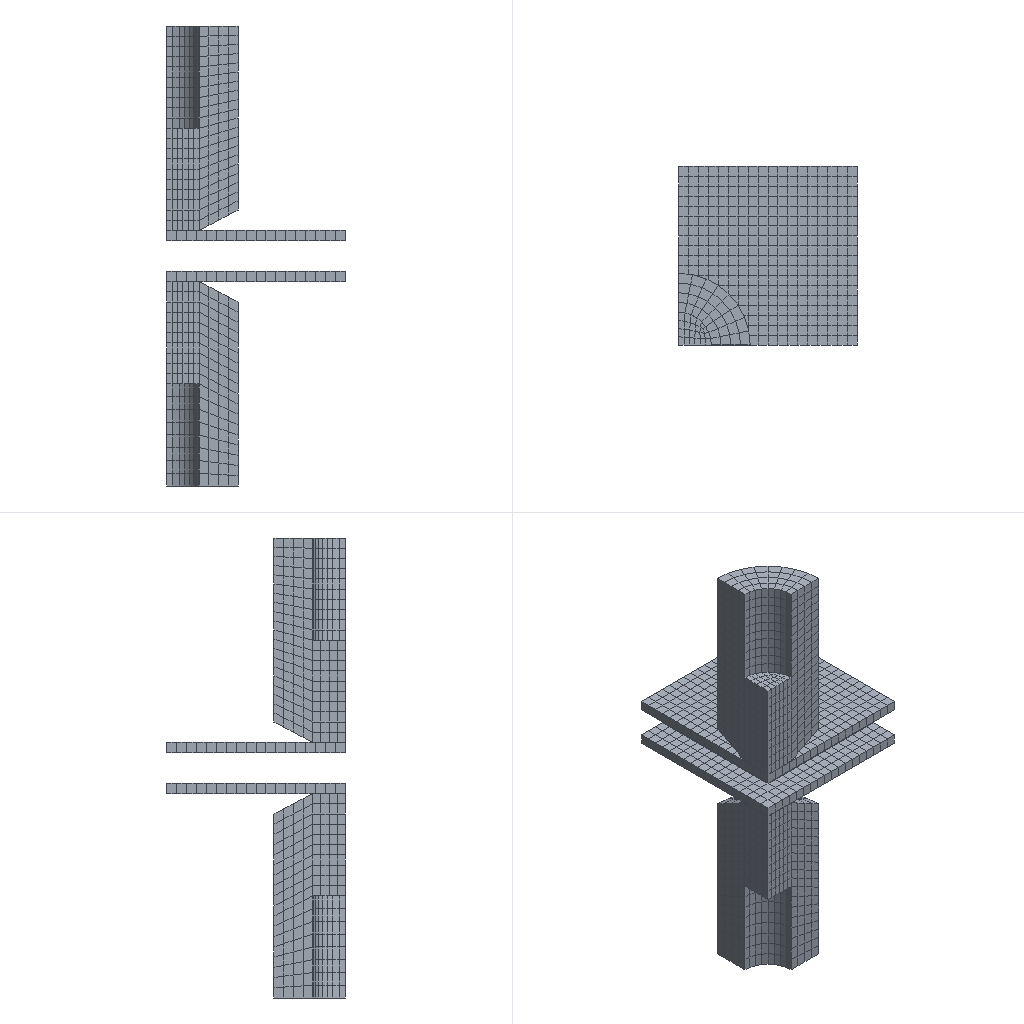Simulation study | abaqus
Set-up summary:
category,name,step,type,value,unit,region
solver,abaqus
solver,version,,,Abaqus/Standard 2020
units,not stated in the deck,,not stated
analysis,deck,,coupled temperature-displacement,coupled temperature-displacement
load_step,Step-1,Step-1,coupled temperature-displacement,nlgeom=True
load_step,Step-1-1,Step-1-1,coupled temperature-displacement,nlgeom=True
load_step,Step-2-jiazai,Step-2-jiazai,coupled temperature-displacement,nlgeom=True
load_step,Step-2-2-tongdian,Step-2-2-tongdian,coupled temperature-displacement,nlgeom=True
load_step,Step-2-3-xiezai,Step-2-3-xiezai,coupled temperature-displacement,nlgeom=True
load_step,Step-2-4-duandianbaochi,Step-2-4-duandianbaochi,coupled temperature-displacement,nlgeom=True
contact,interactions,,,general=0 pairs=3 ties=0
load_step,requested,,,6
mesh,nodes,,,3772
mesh,elements,,,2324
element_type,Q3D8R,,solid,2324
load,load commands in deck,,count,4
bc,support commands in deck,,count,25
material,CU_ELEC,,in results
material,FE_STEEL,,in results
check,setup vs results,,match,"per instance, exact: element labels, types and connectivity; labels of the nodes the elements use; coordinates of those nodes at SINGLE_PRECISION in 4 of 4 instance(s)"
Abaqus input file, long lists of numbers shortened:
*Heading
** Job name: Job-1 Model name: Job-model
** Generated by: Abaqus/CAE 2020
*Preprint, echo=NO, model=NO, history=NO, contact=NO
**
** PARTS
**
*Part, name=work-1
*Node
      1,           0.,   3.2,          14.
      2,           0.,           0.,          14.
** (1207 more lines like these left out)
*Element, type=Q3D8R
  1, 201, 202, 691, 684,  15,  16, 160, 159
  2, 202, 203, 692, 691,  16,  17, 161, 160
** (868 more lines like these left out)
*Nset, nset=Set-2, generate
    1,  1209,     1
*Elset, elset=Set-2, generate
   1,  870,    1
** Section: Section-2-SET-1
*Solid Section, elset=Set-2, material=CU_ELEC
,
*End Part
**
*Part, name=work-2
*Node
      1,         17.5,         17.5,           4.
      2,         17.5,         17.5,           3.
** (720 more lines like these left out)
*Element, type=Q3D8R
  1,  39,  40,  42,  41,   1,   2,   4,   3
  2,  41,  42,  44,  43,   3,   4,   6,   5
** (322 more lines like these left out)
*Nset, nset=Set-1, generate
   1,  722,    1
*Elset, elset=Set-1, generate
   1,  324,    1
** Section: Section-1-SET-1
*Solid Section, elset=Set-1, material=FE_STEEL
,
*End Part
**
*Part, name=work-3
*Node
      1,         17.5,         17.5,          -1.
      2,   16.528,         17.5,          -1.
** (720 more lines like these left out)
*Element, type=Q3D8R
  1,  39,  40,  59,  58,   1,   2,  21,  20
  2,  40,  41,  60,  59,   2,   3,  22,  21
** (322 more lines like these left out)
*Nset, nset=Set-1, generate
   1,  722,    1
*Elset, elset=Set-1, generate
   1,  324,    1
** Section: Section-1-SET-1
*Solid Section, elset=Set-1, material=FE_STEEL
,
*End Part
**
*Part, name=work-4
*Node
      1,           0.,   3.2,          -1.
      2,           0.,           0.,          -1.
** (1117 more lines like these left out)
*Element, type=Q3D8R
  1, 193, 194, 643, 636,  15,  16, 152, 151
  2, 194, 195, 644, 643,  16,  17, 153, 152
** (804 more lines like these left out)
*Nset, nset=Set-2, generate
    1,  1119,     1
*Elset, elset=Set-2, generate
   1,  806,    1
** Section: Section-4-SET-1
*Solid Section, elset=Set-2, material=CU_ELEC
,
*End Part
**
**
** ASSEMBLY
**
*Assembly, name=Assembly
**
*Instance, name=work-1-1, part=work-1
*End Instance
**
*Instance, name=work-2-1, part=work-2
*End Instance
**
*Instance, name=work-3-1, part=work-3
*End Instance
**
*Instance, name=work-4-1, part=work-4
*End Instance
**
*Nset, nset=Set-20, instance=work-1-1
   8,   9,  10,  11,  92,  93,  94, 111, 112, 113, 114, 115, 116, 117, 118, 119
 120, 121, 122, 123, 124, 134, 135, 136, 592, 593, 594, 595, 596, 597, 598, 599
** (1 more lines like these left out)
*Elset, elset=Set-20, instance=work-1-1
 307, 308, 309, 310, 387, 388, 389, 390, 467, 468, 469, 470, 547, 548, 549, 550
 627, 628, 629, 630, 707, 708, 709, 710, 787, 788, 789, 790, 867, 868, 869, 870
*Nset, nset=Set-21, instance=work-1-1
   2,   3,   5,   6,   7,   8,   9,  32,  33,  34,  35,  36,  37,  38,  39,  40
  41,  42,  43,  44,  45,  46,  47,  48,  49,  50,  51,  52,  53,  54,  65,  66
** (9 more lines like these left out)
*Nset, nset=Set-21, instance=work-2-1, generate
 685,  722,    1
*Nset, nset=Set-21, instance=work-4-1
   2,   3,   5,   6,   7,   8,   9,  32,  33,  34,  35,  36,  37,  38,  39,  40
  41,  42,  43,  44,  45,  46,  47,  48,  49,  50,  51,  52,  53,  54,  65,  66
** (9 more lines like these left out)
*Nset, nset=Set-21, instance=work-3-1, generate
 685,  722,    1
*Elset, elset=Set-21, instance=work-1-1
  28,  31,  34,  37,  40,  43,  46,  49,  52,  55,  58,  61,  64,  67,  70,  73
  76,  79,  82,  85,  88,  91,  94,  97, 100, 101, 104, 107, 110, 113, 143, 146
** (7 more lines like these left out)
*Elset, elset=Set-21, instance=work-2-1, generate
 307,  324,    1
*Elset, elset=Set-21, instance=work-4-1
  28,  31,  34,  37,  40,  43,  46,  49,  52,  55,  58,  61,  64,  67,  70,  73
  76,  79,  82,  85,  88,  91,  94,  97, 100, 101, 104, 107, 110, 113, 143, 146
** (7 more lines like these left out)
*Elset, elset=Set-21, instance=work-3-1, generate
 307,  324,    1
*Nset, nset=Set-22, instance=work-1-1
   1,   2,   4,   5,  10,  11,  12,  20,  21,  22,  23,  24,  25,  26,  27,  28
  29,  30,  31,  37,  38,  39,  40,  41,  42,  43,  44,  45,  55,  56,  57, 125
** (8 more lines like these left out)
*Nset, nset=Set-22, instance=work-2-1
  37,  38,  75,  76, 113, 114, 151, 152, 189, 190, 227, 228, 265, 266, 303, 304
 341, 342, 379, 380, 417, 418, 455, 456, 493, 494, 531, 532, 569, 570, 607, 608
** (1 more lines like these left out)
*Nset, nset=Set-22, instance=work-4-1
   1,   2,   4,   5,  10,  11,  12,  20,  21,  22,  23,  24,  25,  26,  27,  28
  29,  30,  31,  37,  38,  39,  40,  41,  42,  43,  44,  45,  55,  56,  57, 121
** (7 more lines like these left out)
*Nset, nset=Set-22, instance=work-3-1, generate
  19,  722,   19
*Elset, elset=Set-22, instance=work-1-1
   5,  10,  15,  20,  25,  26,  27,  28,  41,  42,  43,  56,  57,  58,  71,  72
  73,  86,  87,  88, 116, 117, 118, 119, 120, 141, 142, 143, 144, 145, 146, 147
** (6 more lines like these left out)
*Elset, elset=Set-22, instance=work-2-1, generate
  18,  324,   18
*Elset, elset=Set-22, instance=work-4-1
   5,  10,  15,  20,  25,  26,  27,  28,  41,  42,  43,  56,  57,  58,  71,  72
  73,  86,  87,  88, 116, 117, 118, 119, 120, 141, 142, 143, 144, 145, 146, 147
** (5 more lines like these left out)
*Elset, elset=Set-22, instance=work-3-1, generate
  18,  324,   18
*Nset, nset=Set-23, instance=work-2-1
   1,   2,  39,  40,  77,  78, 115, 116, 153, 154, 191, 192, 229, 230, 267, 268
 305, 306, 343, 344, 381, 382, 419, 420, 457, 458, 495, 496, 533, 534, 571, 572
** (1 more lines like these left out)
*Nset, nset=Set-23, instance=work-3-1, generate
   1,  704,   19
*Elset, elset=Set-23, instance=work-2-1, generate
   1,  307,   18
*Elset, elset=Set-23, instance=work-3-1, generate
   1,  307,   18
*Nset, nset=Set-24, instance=work-2-1, generate
  1,  38,   1
*Nset, nset=Set-24, instance=work-3-1, generate
  1,  38,   1
*Elset, elset=Set-24, instance=work-2-1, generate
  1,  18,   1
*Elset, elset=Set-24, instance=work-3-1, generate
  1,  18,   1
*Nset, nset=Set-25, instance=work-4-1
   7,   8,  11,  12,  77,  78,  79, 100, 101, 102, 103, 104, 105, 106, 107, 108
 109, 110, 111, 112, 113, 141, 142, 143, 467, 468, 469, 470, 471, 472, 473, 474
** (1 more lines like these left out)
*Elset, elset=Set-25, instance=work-4-1, generate
 248,  806,   18
*Nset, nset=Set-26, instance=work-1-1
   8,   9,  10,  11,  92,  93,  94, 111, 112, 113, 114, 115, 116, 117, 118, 119
 120, 121, 122, 123, 124, 134, 135, 136, 592, 593, 594, 595, 596, 597, 598, 599
** (1 more lines like these left out)
*Elset, elset=Set-26, instance=work-1-1
 307, 308, 309, 310, 387, 388, 389, 390, 467, 468, 469, 470, 547, 548, 549, 550
 627, 628, 629, 630, 707, 708, 709, 710, 787, 788, 789, 790, 867, 868, 869, 870
*Nset, nset=Set-27, instance=work-1-1
   8,   9,  10,  11,  92,  93,  94, 111, 112, 113, 114, 115, 116, 117, 118, 119
 120, 121, 122, 123, 124, 134, 135, 136, 592, 593, 594, 595, 596, 597, 598, 599
** (1 more lines like these left out)
*Nset, nset=Set-27, instance=work-4-1
   7,   8,  11,  12,  77,  78,  79, 100, 101, 102, 103, 104, 105, 106, 107, 108
 109, 110, 111, 112, 113, 141, 142, 143, 467, 468, 469, 470, 471, 472, 473, 474
** (1 more lines like these left out)
*Elset, elset=Set-27, instance=work-1-1
 307, 308, 309, 310, 387, 388, 389, 390, 467, 468, 469, 470, 547, 548, 549, 550
 627, 628, 629, 630, 707, 708, 709, 710, 787, 788, 789, 790, 867, 868, 869, 870
*Elset, elset=Set-27, instance=work-4-1, generate
 248,  806,   18
*Nset, nset=Set-28, instance=work-2-1
   1,   2,   3,   4,   5,   6,   7,   8,   9,  10,  11,  12,  13,  14,  15,  16
  17,  18,  19,  20,  21,  22,  23,  24,  25,  26,  27,  28,  29,  30,  31,  32
** (3 more lines like these left out)
*Nset, nset=Set-28, instance=work-3-1
   1,   2,   3,   4,   5,   6,   7,   8,   9,  10,  11,  12,  13,  14,  15,  16
  17,  18,  19,  20,  21,  22,  23,  24,  25,  26,  27,  28,  29,  30,  31,  32
** (3 more lines like these left out)
*Elset, elset=Set-28, instance=work-2-1
   1,   2,   3,   4,   5,   6,   7,   8,   9,  10,  11,  12,  13,  14,  15,  16
  17,  18,  19,  37,  55,  73,  91, 109, 127, 145, 163, 181, 199, 217, 235, 253
** (1 more lines like these left out)
*Elset, elset=Set-28, instance=work-3-1
   1,   2,   3,   4,   5,   6,   7,   8,   9,  10,  11,  12,  13,  14,  15,  16
  17,  18,  19,  37,  55,  73,  91, 109, 127, 145, 163, 181, 199, 217, 235, 253
** (1 more lines like these left out)
*Nset, nset=Set-29, instance=work-1-1, generate
    1,  1209,     1
*Nset, nset=Set-29, instance=work-2-1, generate
   1,  722,    1
*Nset, nset=Set-29, instance=work-4-1, generate
    1,  1119,     1
*Nset, nset=Set-29, instance=work-3-1, generate
   1,  722,    1
*Elset, elset=Set-29, instance=work-1-1, generate
   1,  870,    1
*Elset, elset=Set-29, instance=work-2-1, generate
   1,  324,    1
*Elset, elset=Set-29, instance=work-4-1, generate
   1,  806,    1
*Elset, elset=Set-29, instance=work-3-1, generate
   1,  324,    1
*Nset, nset=Set-30, instance=work-1-1
   1,   2,   3,  13,  14,  15,  16,  17,  18,  19,  20,  21,  22,  32,  33,  34
  35,  36, 159, 160, 161, 162, 163, 164, 165, 166, 167, 168, 169, 170, 171, 172
** (1 more lines like these left out)
*Elset, elset=Set-30, instance=work-1-1
   1,   2,   3,   4,   5,  26,  27,  28,  29,  30,  31,  32,  33,  34,  35,  36
  37,  38,  39,  40, 101, 102, 103
*Nset, nset=Set-31, instance=work-4-1
   4,   5,   6,  55,  56,  57,  58,  59,  60,  61,  62,  63,  64,  65,  66,  67
  68,  69, 301, 302, 303, 304, 305, 306, 307, 308, 309, 310, 311, 312, 313, 314
** (1 more lines like these left out)
*Elset, elset=Set-31, instance=work-4-1
 120, 125, 130, 135, 140, 141, 142, 143, 156, 157, 158, 171, 172, 173, 186, 187
 188, 201, 202, 203, 220, 225, 230
*Elset, elset=_Surf-6_S3, internal, instance=work-1-1
 307, 308, 309, 310, 387, 388, 389, 390, 467, 468, 469, 470, 547, 548, 549, 550
 627, 628, 629, 630, 707, 708, 709, 710, 787, 788, 789, 790, 867, 868, 869, 870
*Surface, type=ELEMENT, name=Surf-6
_Surf-6_S3, S3
*Elset, elset=_Surf-13_S3, internal, instance=work-1-1
 307, 308, 309, 310, 387, 388, 389, 390, 467, 468, 469, 470, 547, 548, 549, 550
 627, 628, 629, 630, 707, 708, 709, 710, 787, 788, 789, 790, 867, 868, 869, 870
*Elset, elset=_Surf-13_S4, internal, instance=work-4-1, generate
 248,  806,   18
*Surface, type=ELEMENT, name=Surf-13
_Surf-13_S3, S3
_Surf-13_S4, S4
*Elset, elset=_m_Surf-7_S4, internal, instance=work-2-1, generate
   1,  324,    1
*Surface, type=ELEMENT, name=m_Surf-7
_m_Surf-7_S4, S4
*Elset, elset=_m_Surf-9_S4, internal, instance=work-1-1
 120, 125, 130, 135, 140, 220, 225, 230
*Elset, elset=_m_Surf-9_S3, internal, instance=work-1-1
 141, 142, 143, 156, 157, 158, 171, 172, 173, 186, 187, 188, 201, 202, 203
*Elset, elset=_m_Surf-9_S5, internal, instance=work-1-1
 231, 232, 233, 234, 311, 312, 313, 314, 391, 392, 393, 394, 471, 472, 473, 474
 551, 552, 553, 554, 631, 632, 633, 634, 711, 712, 713, 714, 791, 792, 793, 794
*Surface, type=ELEMENT, name=m_Surf-9
_m_Surf-9_S4, S4
_m_Surf-9_S3, S3
_m_Surf-9_S5, S5
*Elset, elset=_m_Surf-11_S2, internal, instance=work-4-1
   1,   2,   3,   4,   5,  26,  27,  28,  29,  30,  31,  32,  33,  34,  35,  36
  37,  38,  39,  40, 101, 102, 103
*Elset, elset=_m_Surf-11_S6, internal, instance=work-4-1, generate
 231,  789,   18
*Surface, type=ELEMENT, name=m_Surf-11
_m_Surf-11_S2, S2
_m_Surf-11_S6, S6
*Elset, elset=_s_Surf-7_S5, internal, instance=work-3-1, generate
   1,  324,    1
*Surface, type=ELEMENT, name=s_Surf-7
_s_Surf-7_S5, S5
*Elset, elset=_s_Surf-9_S6, internal, instance=work-2-1, generate
   1,  324,    1
*Surface, type=ELEMENT, name=s_Surf-9
_s_Surf-9_S6, S6
*Elset, elset=_s_Surf-11_S3, internal, instance=work-3-1, generate
   1,  324,    1
*Surface, type=ELEMENT, name=s_Surf-11
_s_Surf-11_S3, S3
*End Assembly
*Amplitude, name=CURRENT_SHIJIA
             0.,              0.,            0.01,              1.
*Amplitude, name=CURRENT_XIEZAI
             0.,              1.,            0.01,              0.
*Amplitude, name=FORCE_SHIJIA
             0.,              0.,             0.1,              1.
*Amplitude, name=FORCE_XIEZAI
             0.,              1.,             0.1,              0.
**
** MATERIALS
**
*Material, name=CU_ELEC
*Conductivity
  385.,  25.
 368.5, 100.
 358.3, 210.
 342.1, 310.
 331.5, 430.
 319.6, 520.
 306.4, 630.
 298.1, 730.
 291.2, 850.
 288.6, 940.
 286.7,1030.
 282.5,1380.
*Density
 8.9e-09,
*Elastic
115000., 0.35,  20.
106000., 0.35, 150.
 99000., 0.36, 350.
 95000., 0.37, 450.
 87000., 0.37, 550.
 76000., 0.39, 650.
 71000., 0.39, 730.
*Electrical Conductivity
 28.41,  25.
   25., 110.
 18.75, 210.
 14.85, 310.
 13.32, 420.
 12.38, 530.
  9.02, 640.
  3.92, 750.
   3.4, 830.
  2.88, 950.
  2.37,1100.
  4.31,1220.
  3.92,1400.
*Expansion
 1.63e-05, 20.
 1.73e-05,150.
  1.8e-05,350.
 1.81e-05,450.
 1.86e-05,550.
 1.88e-05,650.
 1.94e-05,730.
*Joule Heat Fraction
         0.7,
*Plastic
233.,  0., 20.
188.,  0.,150.
130.,  0.,350.
125.,  0.,450.
107.,  0.,550.
 88.,  0.,650.
 50.,  0.,730.
*Specific Heat
 3.8e+08,  25.
 3.9e+08, 100.
   4e+08, 210.
 4.1e+08, 310.
 4.3e+08, 430.
 4.3e+08, 520.
 4.5e+08, 630.
 4.6e+08, 730.
 4.8e+08, 850.
 4.9e+08, 940.
 5.1e+08,1030.
 5.3e+08,1380.
*Material, name=FE_STEEL
*Conductivity
  15.6,  25.
 16.53, 100.
 17.89, 210.
 19.13, 310.
 20.62, 430.
 21.73, 520.
 23.09, 630.
 24.33, 730.
 25.81, 850.
 26.87, 940.
  27.9,1030.
 32.42,1380.
*Density
 7.8e-09,
*Elastic
205000.,  0.3,  20.
182000.,  0.3, 150.
169000.,  0.3, 350.
151000.,  0.3, 550.
121000.,  0.3, 750.
 75000.,  0.3, 950.
 46000.,  0.3,1300.
*Electrical Conductivity
 1.61,  25.
 1.33, 110.
 1.14, 210.
 1.01, 310.
 0.91, 420.
 0.84, 530.
 0.78, 640.
 0.74, 750.
 0.71, 830.
 0.68, 950.
 0.64,1100.
 0.62,1220.
  0.6,1400.
*Expansion
 2.023e-05,  20.
 2.046e-05, 150.
 2.087e-05, 350.
  2.13e-05, 550.
 2.178e-05, 750.
 2.238e-05, 950.
 2.341e-05,1300.
*Joule Heat Fraction
          1.,
*Plastic
300.,   0.,  20.
223.,   0., 150.
173.,   0., 350.
126.,   0., 550.
 95.,   0., 750.
 54.,   0., 950.
 32.,   0.,1300.
*Specific Heat
 4.6e+08,  25.
 4.8e+08, 100.
   5e+08, 210.
 5.2e+08, 310.
 5.4e+08, 430.
 5.5e+08, 520.
 5.7e+08, 630.
 5.9e+08, 730.
 6.1e+08, 850.
 6.8e+08, 940.
 6.5e+08,1030.
 8.8e+08,1380.
**
** INTERACTION PROPERTIES
**
*Surface Interaction, name=BAN_BAN
1.,
*Friction, slip tolerance=0.005
 0.2,
*Surface Behavior, pressure-overclosure=HARD
*Gap Conductance
140.,    0.,   20.
  0., 0.001,   20.
150.,    0.,  205.
  0., 0.001,  205.
160.,    0.,  650.
  0., 0.001,  650.
160.,    0.,  870.
  0., 0.001,  870.
*Gap Heat Generation
1., 0.5
*Gap Electrical Conductance
100.,   0.
  0., 0.01
*Surface Interaction, name=DJ_BAN
1.,
*Friction, slip tolerance=0.005
 0.2,
*Surface Behavior, pressure-overclosure=HARD
*Gap Conductance
 560.,    0.,   20.
   0., 0.001,   20.
 640.,    0.,  205.
   0., 0.001,  205.
1300.,    0.,  650.
   0., 0.001,  650.
4800.,    0.,  870.
   0., 0.001,  870.
*Gap Heat Generation
1., 0.5
*Gap Electrical Conductance
100.,   0.
  0., 0.01
**
** PHYSICAL CONSTANTS
**
*Physical Constants, absolute zero=-273.15, stefan boltzmann=5.67e-11
**
** BOUNDARY CONDITIONS
**
** Name: Disp-BC-1 Type: 对称/反对称/完全固定
*Boundary
Set-21, YSYMM
** Name: Disp-BC-2 Type: 对称/反对称/完全固定
*Boundary
Set-22, XSYMM
** Name: Disp-BC-3 Type: 位移/转角
*Boundary
Set-27, 1, 1
** Name: Disp-BC-8 Type: 位移/转角
*Boundary
Set-28, 1, 1
**
** PREDEFINED FIELDS
**
** Name: Predefined Field-1   Type: Temperature
*Initial Conditions, type=TEMPERATURE
Set-29, 20.
**
** INTERACTIONS
**
** Interaction: BAN_BAN-1
*Contact Pair, interaction=BAN_BAN, type=SURFACE TO SURFACE
s_Surf-7, m_Surf-7
** Interaction: Int-6
*Contact Pair, interaction=DJ_BAN, type=SURFACE TO SURFACE
m_Surf-9, s_Surf-9
** Interaction: Int-7
*Contact Pair, interaction=DJ_BAN, type=SURFACE TO SURFACE
s_Surf-11, m_Surf-11
** ----------------------------------------------------------------
**
** STEP: Step-1
**
*Step, name=Step-1, nlgeom=YES, inc=10000
*Coupled Temperature-displacement, electrical, creep=none, deltmx=1e+09
0.0015, 0.15, 1.5e-08, 0.015
**
** BOUNDARY CONDITIONS
**
** Name: Disp-BC-3 Type: 位移/转角
*Boundary
Set-27, 2, 2
Set-27, 4, 4
Set-27, 5, 5
Set-27, 6, 6
** Name: Disp-BC-8 Type: 位移/转角
*Boundary
Set-28, 2, 2
Set-28, 3, 3
**
** LOADS
**
** Name: Load-1   Type: Pressure
*Dsload, amplitude=FORCE_SHIJIA
Surf-13, P, 36.492
**
** OUTPUT REQUESTS
**
*Restart, write, frequency=0
**
** FIELD OUTPUT: F-Output-1
**
*Output, field
*Node Output
CECHG, CECUR, CF, EPOT, NT, RCHG, RECUR, RF
RFL, RM, RT, TF, U
*Element Output, directions=YES
E, ECD, EFLX, EPG, HFL, LE, MISES, MISESMAX, MISESONLY, NCURS, NE, P, PE, PEEQ, PEEQMAX, PEEQT
PEMAG, PRESSONLY, S, SEQUT, SF, SSAVG, TEMP, VEEQ, YIELDPOT
*Contact Output
CDISP, CSTRESS, ECD, ECDA, ECDT, ECDTA
*Radiation Output
FTEMP,
**
** HISTORY OUTPUT: H-Output-1
**
*Output, history, variable=PRESELECT
*End Step
** ----------------------------------------------------------------
**
** STEP: Step-1-1
**
*Step, name=Step-1-1, nlgeom=YES
*Coupled Temperature-displacement, electrical, creep=none, deltmx=1e+09
0.01, 0.3, 3e-06, 0.1
**
** LOADS
**
** Name: Load-1   Type: Pressure
**
** OUTPUT REQUESTS
**
*Restart, write, frequency=0
**
** FIELD OUTPUT: F-Output-1
**
*Output, field
*Node Output
CECHG, CECUR, CF, EPOT, NT, RCHG, RECUR, RF
RFL, RM, RT, TF, U
*Element Output, directions=YES
E, ECD, EFLX, EPG, HFL, LE, MISES, MISESMAX, MISESONLY, NCURS, NE, P, PE, PEEQ, PEEQMAX, PEEQT
PEMAG, PRESSONLY, S, SEQUT, SF, SSAVG, TEMP, VEEQ, YIELDPOT
*Contact Output
CDISP, CSTRESS, ECD, ECDA, ECDT, ECDTA
*Radiation Output
FTEMP,
**
** HISTORY OUTPUT: H-Output-1
**
*Output, history, variable=PRESELECT
*End Step
** ----------------------------------------------------------------
**
** STEP: Step-2-jiazai
**
*Step, name=Step-2-jiazai, nlgeom=YES, inc=10000
*Coupled Temperature-displacement, electrical, creep=none, deltmx=1e+08
0.001, 0.01, 2e-08, 0.003
**
** BOUNDARY CONDITIONS
**
** Name: BC-6 Type: 电势
*Boundary, amplitude=CURRENT_SHIJIA
Set-30, 9, 9, 100.
** Name: Elec-BC-1 Type: 电势
*Boundary
Set-31, 9, 9
**
** LOADS
**
** Name: Load-1   Type: Pressure
**
** OUTPUT REQUESTS
**
*Restart, write, frequency=0
**
** FIELD OUTPUT: F-Output-1
**
*Output, field
*Node Output
CECHG, CECUR, CF, EPOT, NT, RCHG, RECUR, RF
RFL, RM, RT, TF, U
*Element Output, directions=YES
E, ECD, EFLX, EPG, HFL, LE, MISES, MISESMAX, MISESONLY, NCURS, NE, P, PE, PEEQ, PEEQMAX, PEEQT
PEMAG, PRESSONLY, S, SEQUT, SF, SSAVG, TEMP, VEEQ, YIELDPOT
*Contact Output
CDISP, CSTRESS, ECD, ECDA, ECDT, ECDTA
*Radiation Output
FTEMP,
**
** HISTORY OUTPUT: H-Output-1
**
*Output, history, variable=PRESELECT
*End Step
** ----------------------------------------------------------------
**
** STEP: Step-2-2-tongdian
**
*Step, name=Step-2-2-tongdian, nlgeom=YES
*Coupled Temperature-displacement, electrical, creep=none, deltmx=1e+07
0.017, 0.17, 1.7e-06, 0.17
**
** BOUNDARY CONDITIONS
**
** Name: BC-6 Type: 电势
*Boundary, op=NEW
Set-30, 9, 9, 100.
** Name: Disp-BC-1 Type: 对称/反对称/完全固定
*Boundary, op=NEW
Set-21, YSYMM
** Name: Disp-BC-2 Type: 对称/反对称/完全固定
*Boundary, op=NEW
Set-22, XSYMM
** Name: Disp-BC-3 Type: 位移/转角
*Boundary, op=NEW
Set-27, 1, 1
Set-27, 2, 2
Set-27, 4, 4
Set-27, 5, 5
Set-27, 6, 6
** Name: Disp-BC-8 Type: 位移/转角
*Boundary, op=NEW
Set-28, 1, 1
Set-28, 2, 2
Set-28, 3, 3
** Name: Elec-BC-1 Type: 电势
*Boundary, op=NEW
Set-31, 9, 9
**
** OUTPUT REQUESTS
**
*Restart, write, frequency=0
**
** FIELD OUTPUT: F-Output-1
**
*Output, field
*Node Output
CECHG, CECUR, CF, EPOT, NT, RCHG, RECUR, RF
RFL, RM, RT, TF, U
*Element Output, directions=YES
E, ECD, EFLX, EPG, HFL, LE, MISES, MISESMAX, MISESONLY, NCURS, NE, P, PE, PEEQ, PEEQMAX, PEEQT
PEMAG, PRESSONLY, S, SEQUT, SF, SSAVG, TEMP, VEEQ, YIELDPOT
*Contact Output
CDISP, CSTRESS, ECD, ECDA, ECDT, ECDTA
*Radiation Output
FTEMP,
**
** HISTORY OUTPUT: H-Output-1
**
*Output, history, variable=PRESELECT
*End Step
** ----------------------------------------------------------------
**
** STEP: Step-2-3-xiezai
**
*Step, name=Step-2-3-xiezai, nlgeom=YES
*Coupled Temperature-displacement, electrical, creep=none, deltmx=1e+07
0.001, 0.01, 1e-07, 0.01
**
** BOUNDARY CONDITIONS
**
** Name: BC-6 Type: 电势
*Boundary, amplitude=CURRENT_XIEZAI
Set-30, 9, 9, 100.
**
** OUTPUT REQUESTS
**
*Restart, write, frequency=0
**
** FIELD OUTPUT: F-Output-1
**
*Output, field
*Node Output
CECHG, CECUR, CF, EPOT, NT, RCHG, RECUR, RF
RFL, RM, RT, TF, U
*Element Output, directions=YES
E, ECD, EFLX, EPG, HFL, LE, MISES, MISESMAX, MISESONLY, NCURS, NE, P, PE, PEEQ, PEEQMAX, PEEQT
PEMAG, PRESSONLY, S, SEQUT, SF, SSAVG, TEMP, VEEQ, YIELDPOT
*Contact Output
CDISP, CSTRESS, ECD, ECDA, ECDT, ECDTA
*Radiation Output
FTEMP,
**
** HISTORY OUTPUT: H-Output-1
**
*Output, history, variable=PRESELECT
*End Step
** ----------------------------------------------------------------
**
** STEP: Step-2-4-duandianbaochi
**
*Step, name=Step-2-4-duandianbaochi, nlgeom=YES
*Coupled Temperature-displacement, electrical, creep=none, deltmx=1e+09
0.006, 0.6, 6e-06, 0.06
**
** OUTPUT REQUESTS
**
*Restart, write, frequency=0
**
** FIELD OUTPUT: F-Output-1
**
*Output, field
*Node Output
CECHG, CECUR, CF, EPOT, NT, RCHG, RECUR, RF
RFL, RM, RT, TF, U
*Element Output, directions=YES
E, ECD, EFLX, EPG, HFL, LE, MISES, MISESMAX, MISESONLY, NCURS, NE, P, PE, PEEQ, PEEQMAX, PEEQT
PEMAG, PRESSONLY, S, SEQUT, SF, SSAVG, TEMP, VEEQ, YIELDPOT
*Contact Output
CDISP, CSTRESS, ECD, ECDA, ECDT, ECDTA
*Radiation Output
FTEMP,
**
** HISTORY OUTPUT: H-Output-1
**
*Output, history, variable=PRESELECT
*End Step
Results summary:
result,step,,completed,increments=30 time=0.15/0.15
result,step,,completed,increments=8 time=0.3/0.3
result,step,,completed,increments=6 time=0.01/0.01
result,step,,completed,increments=6 time=0.17/0.17
result,step,,completed,increments=6 time=0.01/0.01
result,step,,partial,increments=16 time=0.6/0.6
result,analysis,,,"coupled temperature-displacement, steady state"
result,last_loadstep,,,6
result,analysis steps,,count,6
result,primary field,,,"U, NT11"
result,reaction total,,FX,-0.2868,model units
result,reaction total,,FY,-0.2911,model units
result,reaction total,,FZ,-0.000391,model units